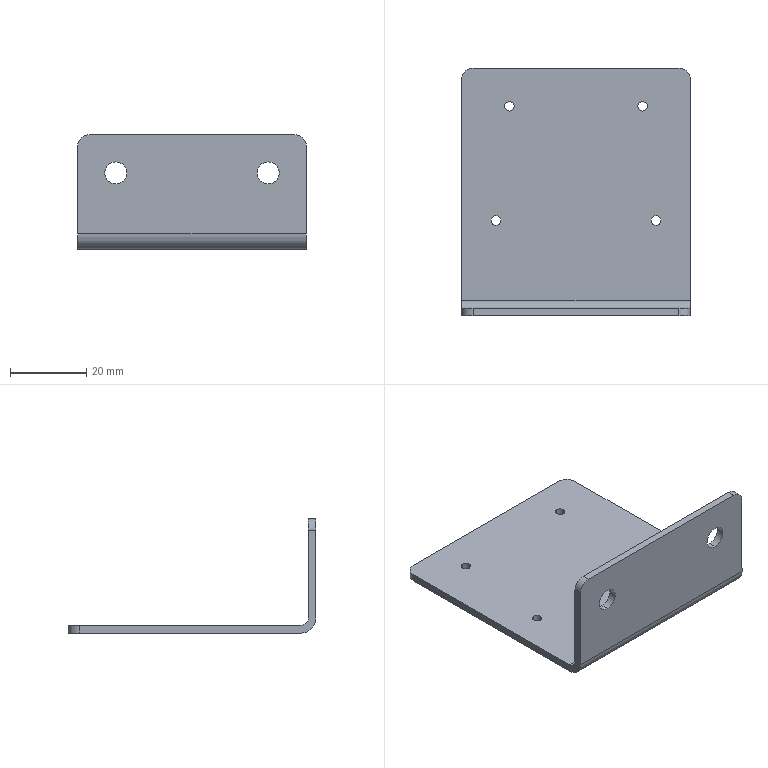Part | STEP file | J452-EBZ05-23-08 | 1 solid | 26 faces | box 60 x 65 x 30 mm | volume 10845 mm3 | cylinder 18 | plane 8 | commonest cylinder face diameters 2.5 x8 5.8 x4 6 x4 4 x1 8 x1